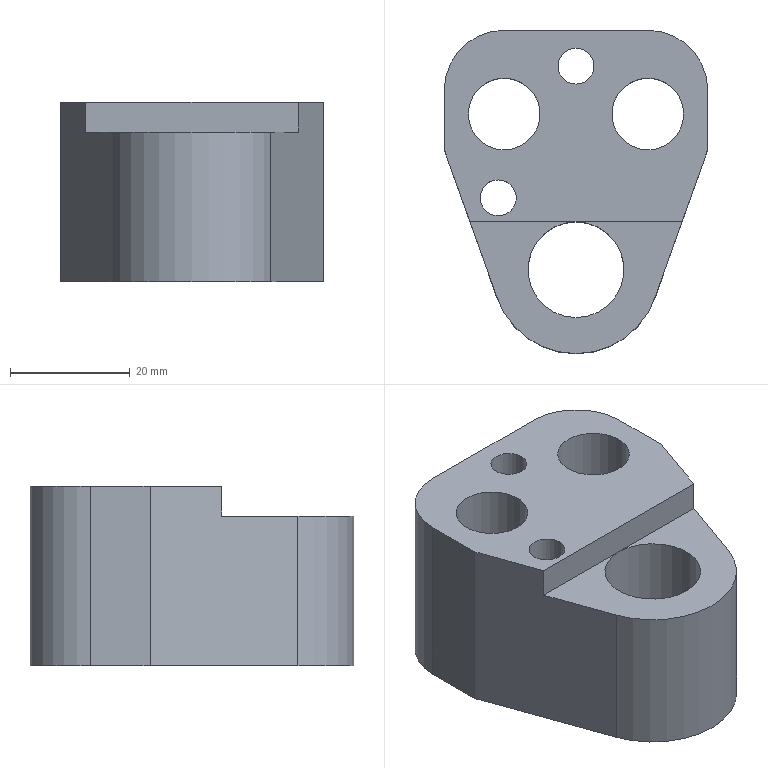Part | NX | features solid 2 | 1 solid | 25 faces | box 44 x 54 x 30 mm | volume 36572 mm3 | plane 13 | cylinder 12 | commonest cylinder face diameters 6 x2 8 x2 12 x2 17 x2 20 x2 16 x1
STEP:
#1=CARTESIAN_POINT('',(278.65,-40.99,61.));
#2=VERTEX_POINT('',#1);
#3=CARTESIAN_POINT('',(278.65,-36.99,61.));
#4=DIRECTION('',(0.,0.,1.));
#5=DIRECTION('',(0.,-1.,0.));
#6=AXIS2_PLACEMENT_3D('',#3,#4,#5);
#7=CIRCLE('',#6,4.);
#8=EDGE_CURVE('',#2,#2,#7,.F.);
#9=ORIENTED_EDGE('',*,*,#8,.F.);
#10=EDGE_LOOP('',(#9));
#11=FACE_BOUND('',#10,.T.);
#12=CARTESIAN_POINT('',(266.65,-36.49,61.));
#13=VERTEX_POINT('',#12);
#14=CARTESIAN_POINT('',(266.65,-44.99,61.));
#15=DIRECTION('',(0.,0.,-1.));
#16=DIRECTION('',(0.,1.,0.));
#17=AXIS2_PLACEMENT_3D('',#14,#15,#16);
#18=CIRCLE('',#17,8.5);
#19=EDGE_CURVE('',#13,#13,#18,.T.);
#20=ORIENTED_EDGE('',*,*,#19,.F.);
#21=EDGE_LOOP('',(#20));
#22=FACE_BOUND('',#21,.T.);
#23=CARTESIAN_POINT('',(290.65,-36.49,61.));
#24=VERTEX_POINT('',#23);
#25=CARTESIAN_POINT('',(290.65,-44.99,61.));
#26=DIRECTION('',(0.,0.,-1.));
#27=DIRECTION('',(0.,1.,0.));
#28=AXIS2_PLACEMENT_3D('',#25,#26,#27);
#29=CIRCLE('',#28,8.5);
#30=EDGE_CURVE('',#24,#24,#29,.T.);
#31=ORIENTED_EDGE('',*,*,#30,.F.);
#32=EDGE_LOOP('',(#31));
#33=FACE_BOUND('',#32,.T.);
#34=CARTESIAN_POINT('',(278.65,-78.99,61.));
#35=VERTEX_POINT('',#34);
#36=CARTESIAN_POINT('',(278.65,-70.99,61.));
#37=DIRECTION('',(0.,0.,1.));
#38=DIRECTION('',(0.,-1.,0.));
#39=AXIS2_PLACEMENT_3D('',#36,#37,#38);
#40=CIRCLE('',#39,8.);
#41=EDGE_CURVE('',#35,#35,#40,.T.);
#42=ORIENTED_EDGE('',*,*,#41,.T.);
#43=EDGE_LOOP('',(#42));
#44=FACE_BOUND('',#43,.T.);
#45=CARTESIAN_POINT('',(291.836,-75.694,61.));
#46=VERTEX_POINT('',#45);
#47=CARTESIAN_POINT('',(300.65,-50.99,61.));
#48=VERTEX_POINT('',#47);
#49=CARTESIAN_POINT('',(291.836,-75.694,61.));
#50=DIRECTION('',(0.336,0.9418,0.));
#51=VECTOR('',#50,1000.);
#52=LINE('',#49,#51);
#53=EDGE_CURVE('',#46,#48,#52,.T.);
#54=ORIENTED_EDGE('',*,*,#53,.F.);
#55=CARTESIAN_POINT('',(265.464,-75.694,61.));
#56=VERTEX_POINT('',#55);
#57=CARTESIAN_POINT('',(278.65,-70.99,61.));
#58=DIRECTION('',(0.,0.,-1.));
#59=DIRECTION('',(0.,1.,0.));
#60=AXIS2_PLACEMENT_3D('',#57,#58,#59);
#61=CIRCLE('',#60,14.);
#62=EDGE_CURVE('',#46,#56,#61,.T.);
#63=ORIENTED_EDGE('',*,*,#62,.T.);
#64=CARTESIAN_POINT('',(256.65,-50.99,61.));
#65=VERTEX_POINT('',#64);
#66=CARTESIAN_POINT('',(265.464,-75.694,61.));
#67=DIRECTION('',(-0.336,0.9418,0.));
#68=VECTOR('',#67,1000.);
#69=LINE('',#66,#68);
#70=EDGE_CURVE('',#56,#65,#69,.T.);
#71=ORIENTED_EDGE('',*,*,#70,.T.);
#72=CARTESIAN_POINT('',(256.65,-40.99,61.));
#73=VERTEX_POINT('',#72);
#74=CARTESIAN_POINT('',(256.65,-50.99,61.));
#75=DIRECTION('',(0.,1.,0.));
#76=VECTOR('',#75,1000.);
#77=LINE('',#74,#76);
#78=EDGE_CURVE('',#65,#73,#77,.T.);
#79=ORIENTED_EDGE('',*,*,#78,.T.);
#80=CARTESIAN_POINT('',(266.65,-30.99,61.));
#81=VERTEX_POINT('',#80);
#82=CARTESIAN_POINT('',(266.65,-40.99,61.));
#83=DIRECTION('',(0.,0.,-1.));
#84=DIRECTION('',(0.,1.,0.));
#85=AXIS2_PLACEMENT_3D('',#82,#83,#84);
#86=CIRCLE('',#85,10.);
#87=EDGE_CURVE('',#73,#81,#86,.T.);
#88=ORIENTED_EDGE('',*,*,#87,.T.);
#89=CARTESIAN_POINT('',(290.65,-30.99,61.));
#90=VERTEX_POINT('',#89);
#91=CARTESIAN_POINT('',(290.65,-30.99,61.));
#92=DIRECTION('',(-1.,0.,0.));
#93=VECTOR('',#92,1000.);
#94=LINE('',#91,#93);
#95=EDGE_CURVE('',#90,#81,#94,.T.);
#96=ORIENTED_EDGE('',*,*,#95,.F.);
#97=CARTESIAN_POINT('',(300.65,-40.99,61.));
#98=VERTEX_POINT('',#97);
#99=CARTESIAN_POINT('',(290.65,-40.99,61.));
#100=DIRECTION('',(0.,0.,-1.));
#101=DIRECTION('',(0.,1.,0.));
#102=AXIS2_PLACEMENT_3D('',#99,#100,#101);
#103=CIRCLE('',#102,10.);
#104=EDGE_CURVE('',#90,#98,#103,.T.);
#105=ORIENTED_EDGE('',*,*,#104,.T.);
#106=CARTESIAN_POINT('',(300.65,-50.99,61.));
#107=DIRECTION('',(0.,1.,0.));
#108=VECTOR('',#107,1000.);
#109=LINE('',#106,#108);
#110=EDGE_CURVE('',#48,#98,#109,.T.);
#111=ORIENTED_EDGE('',*,*,#110,.F.);
#112=EDGE_LOOP('',(#54,#63,#71,#79,#88,#96,#105,#111));
#113=FACE_BOUND('',#112,.T.);
#114=CARTESIAN_POINT('',(265.65,-62.99,61.));
#115=VERTEX_POINT('',#114);
#116=CARTESIAN_POINT('',(265.65,-58.99,61.));
#117=DIRECTION('',(0.,0.,1.));
#118=DIRECTION('',(0.,-1.,0.));
#119=AXIS2_PLACEMENT_3D('',#116,#117,#118);
#120=CIRCLE('',#119,4.);
#121=EDGE_CURVE('',#115,#115,#120,.F.);
#122=ORIENTED_EDGE('',*,*,#121,.F.);
#123=EDGE_LOOP('',(#122));
#124=FACE_BOUND('',#123,.T.);
#125=CARTESIAN_POINT('',(290.65,-40.99,61.));
#126=DIRECTION('',(0.,0.,-1.));
#127=DIRECTION('',(0.,1.,0.));
#128=AXIS2_PLACEMENT_3D('',#125,#126,#127);
#129=PLANE('',#128);
#130=ADVANCED_FACE('',(#11,#22,#33,#44,#113,#124),#129,.T.);
#131=CARTESIAN_POINT('',(278.65,-33.99,91.));
#132=VERTEX_POINT('',#131);
#133=CARTESIAN_POINT('',(278.65,-36.99,91.));
#134=DIRECTION('',(0.,0.,-1.));
#135=DIRECTION('',(0.,1.,0.));
#136=AXIS2_PLACEMENT_3D('',#133,#134,#135);
#137=CIRCLE('',#136,3.);
#138=EDGE_CURVE('',#132,#132,#137,.T.);
#139=ORIENTED_EDGE('',*,*,#138,.F.);
#140=EDGE_LOOP('',(#139));
#141=FACE_BOUND('',#140,.T.);
#142=CARTESIAN_POINT('',(278.65,-33.99,81.));
#143=VERTEX_POINT('',#142);
#144=CARTESIAN_POINT('',(278.65,-36.99,81.));
#145=DIRECTION('',(0.,0.,-1.));
#146=DIRECTION('',(0.,1.,0.));
#147=AXIS2_PLACEMENT_3D('',#144,#145,#146);
#148=CIRCLE('',#147,3.);
#149=EDGE_CURVE('',#143,#143,#148,.T.);
#150=ORIENTED_EDGE('',*,*,#149,.T.);
#151=EDGE_LOOP('',(#150));
#152=FACE_BOUND('',#151,.T.);
#153=CARTESIAN_POINT('',(278.65,-36.99,61.));
#154=DIRECTION('',(0.,0.,1.));
#155=DIRECTION('',(0.,-1.,0.));
#156=AXIS2_PLACEMENT_3D('',#153,#154,#155);
#157=CYLINDRICAL_SURFACE('',#156,3.);
#158=ADVANCED_FACE('',(#141,#152),#157,.F.);
#159=CARTESIAN_POINT('',(266.65,-38.99,91.));
#160=VERTEX_POINT('',#159);
#161=CARTESIAN_POINT('',(266.65,-44.99,91.));
#162=DIRECTION('',(0.,0.,-1.));
#163=DIRECTION('',(0.,1.,0.));
#164=AXIS2_PLACEMENT_3D('',#161,#162,#163);
#165=CIRCLE('',#164,6.);
#166=EDGE_CURVE('',#160,#160,#165,.T.);
#167=ORIENTED_EDGE('',*,*,#166,.F.);
#168=EDGE_LOOP('',(#167));
#169=FACE_BOUND('',#168,.T.);
#170=CARTESIAN_POINT('',(266.65,-38.99,73.));
#171=VERTEX_POINT('',#170);
#172=CARTESIAN_POINT('',(266.65,-44.99,73.));
#173=DIRECTION('',(0.,0.,-1.));
#174=DIRECTION('',(0.,1.,0.));
#175=AXIS2_PLACEMENT_3D('',#172,#173,#174);
#176=CIRCLE('',#175,6.);
#177=EDGE_CURVE('',#171,#171,#176,.T.);
#178=ORIENTED_EDGE('',*,*,#177,.T.);
#179=EDGE_LOOP('',(#178));
#180=FACE_BOUND('',#179,.T.);
#181=CARTESIAN_POINT('',(266.65,-44.99,61.));
#182=DIRECTION('',(0.,0.,1.));
#183=DIRECTION('',(0.,-1.,0.));
#184=AXIS2_PLACEMENT_3D('',#181,#182,#183);
#185=CYLINDRICAL_SURFACE('',#184,6.);
#186=ADVANCED_FACE('',(#169,#180),#185,.F.);
#187=CARTESIAN_POINT('',(290.65,-38.99,91.));
#188=VERTEX_POINT('',#187);
#189=CARTESIAN_POINT('',(290.65,-44.99,91.));
#190=DIRECTION('',(0.,0.,-1.));
#191=DIRECTION('',(0.,1.,0.));
#192=AXIS2_PLACEMENT_3D('',#189,#190,#191);
#193=CIRCLE('',#192,6.);
#194=EDGE_CURVE('',#188,#188,#193,.T.);
#195=ORIENTED_EDGE('',*,*,#194,.F.);
#196=EDGE_LOOP('',(#195));
#197=FACE_BOUND('',#196,.T.);
#198=CARTESIAN_POINT('',(290.65,-38.99,73.));
#199=VERTEX_POINT('',#198);
#200=CARTESIAN_POINT('',(290.65,-44.99,73.));
#201=DIRECTION('',(0.,0.,-1.));
#202=DIRECTION('',(0.,1.,0.));
#203=AXIS2_PLACEMENT_3D('',#200,#201,#202);
#204=CIRCLE('',#203,6.);
#205=EDGE_CURVE('',#199,#199,#204,.T.);
#206=ORIENTED_EDGE('',*,*,#205,.T.);
#207=EDGE_LOOP('',(#206));
#208=FACE_BOUND('',#207,.T.);
#209=CARTESIAN_POINT('',(290.65,-44.99,61.));
#210=DIRECTION('',(0.,0.,1.));
#211=DIRECTION('',(0.,-1.,0.));
#212=AXIS2_PLACEMENT_3D('',#209,#210,#211);
#213=CYLINDRICAL_SURFACE('',#212,6.);
#214=ADVANCED_FACE('',(#197,#208),#213,.F.);
#215=CARTESIAN_POINT('',(265.65,-55.99,91.));
#216=VERTEX_POINT('',#215);
#217=CARTESIAN_POINT('',(265.65,-58.99,91.));
#218=DIRECTION('',(0.,0.,-1.));
#219=DIRECTION('',(0.,1.,0.));
#220=AXIS2_PLACEMENT_3D('',#217,#218,#219);
#221=CIRCLE('',#220,3.);
#222=EDGE_CURVE('',#216,#216,#221,.T.);
#223=ORIENTED_EDGE('',*,*,#222,.T.);
#224=EDGE_LOOP('',(#223));
#225=FACE_BOUND('',#224,.T.);
#226=ORIENTED_EDGE('',*,*,#166,.T.);
#227=EDGE_LOOP('',(#226));
#228=FACE_BOUND('',#227,.T.);
#229=CARTESIAN_POINT('',(260.931,-62.99,91.));
#230=VERTEX_POINT('',#229);
#231=CARTESIAN_POINT('',(256.65,-50.99,91.));
#232=VERTEX_POINT('',#231);
#233=CARTESIAN_POINT('',(265.464,-75.694,91.));
#234=DIRECTION('',(-0.336,0.9418,0.));
#235=VECTOR('',#234,1000.);
#236=LINE('',#233,#235);
#237=EDGE_CURVE('',#230,#232,#236,.T.);
#238=ORIENTED_EDGE('',*,*,#237,.F.);
#239=CARTESIAN_POINT('',(296.368,-62.99,91.));
#240=VERTEX_POINT('',#239);
#241=CARTESIAN_POINT('',(296.368,-62.99,91.));
#242=DIRECTION('',(-1.,0.,0.));
#243=VECTOR('',#242,1000.);
#244=LINE('',#241,#243);
#245=EDGE_CURVE('',#240,#230,#244,.T.);
#246=ORIENTED_EDGE('',*,*,#245,.F.);
#247=CARTESIAN_POINT('',(300.65,-50.99,91.));
#248=VERTEX_POINT('',#247);
#249=CARTESIAN_POINT('',(291.836,-75.694,91.));
#250=DIRECTION('',(0.336,0.9418,0.));
#251=VECTOR('',#250,1000.);
#252=LINE('',#249,#251);
#253=EDGE_CURVE('',#240,#248,#252,.T.);
#254=ORIENTED_EDGE('',*,*,#253,.T.);
#255=CARTESIAN_POINT('',(300.65,-40.99,91.));
#256=VERTEX_POINT('',#255);
#257=CARTESIAN_POINT('',(300.65,-50.99,91.));
#258=DIRECTION('',(0.,1.,0.));
#259=VECTOR('',#258,1000.);
#260=LINE('',#257,#259);
#261=EDGE_CURVE('',#248,#256,#260,.T.);
#262=ORIENTED_EDGE('',*,*,#261,.T.);
#263=CARTESIAN_POINT('',(290.65,-30.99,91.));
#264=VERTEX_POINT('',#263);
#265=CARTESIAN_POINT('',(290.65,-40.99,91.));
#266=DIRECTION('',(0.,0.,-1.));
#267=DIRECTION('',(0.,1.,0.));
#268=AXIS2_PLACEMENT_3D('',#265,#266,#267);
#269=CIRCLE('',#268,10.);
#270=EDGE_CURVE('',#264,#256,#269,.T.);
#271=ORIENTED_EDGE('',*,*,#270,.F.);
#272=CARTESIAN_POINT('',(266.65,-30.99,91.));
#273=VERTEX_POINT('',#272);
#274=CARTESIAN_POINT('',(290.65,-30.99,91.));
#275=DIRECTION('',(-1.,0.,0.));
#276=VECTOR('',#275,1000.);
#277=LINE('',#274,#276);
#278=EDGE_CURVE('',#264,#273,#277,.T.);
#279=ORIENTED_EDGE('',*,*,#278,.T.);
#280=CARTESIAN_POINT('',(256.65,-40.99,91.));
#281=VERTEX_POINT('',#280);
#282=CARTESIAN_POINT('',(266.65,-40.99,91.));
#283=DIRECTION('',(0.,0.,-1.));
#284=DIRECTION('',(0.,1.,0.));
#285=AXIS2_PLACEMENT_3D('',#282,#283,#284);
#286=CIRCLE('',#285,10.);
#287=EDGE_CURVE('',#281,#273,#286,.T.);
#288=ORIENTED_EDGE('',*,*,#287,.F.);
#289=CARTESIAN_POINT('',(256.65,-50.99,91.));
#290=DIRECTION('',(0.,1.,0.));
#291=VECTOR('',#290,1000.);
#292=LINE('',#289,#291);
#293=EDGE_CURVE('',#232,#281,#292,.T.);
#294=ORIENTED_EDGE('',*,*,#293,.F.);
#295=EDGE_LOOP('',(#238,#246,#254,#262,#271,#279,#288,#294));
#296=FACE_BOUND('',#295,.T.);
#297=ORIENTED_EDGE('',*,*,#194,.T.);
#298=EDGE_LOOP('',(#297));
#299=FACE_BOUND('',#298,.T.);
#300=ORIENTED_EDGE('',*,*,#138,.T.);
#301=EDGE_LOOP('',(#300));
#302=FACE_BOUND('',#301,.T.);
#303=CARTESIAN_POINT('',(290.65,-40.99,91.));
#304=DIRECTION('',(0.,0.,-1.));
#305=DIRECTION('',(0.,1.,0.));
#306=AXIS2_PLACEMENT_3D('',#303,#304,#305);
#307=PLANE('',#306);
#308=ADVANCED_FACE('',(#225,#228,#296,#299,#302),#307,.F.);
#309=CARTESIAN_POINT('',(296.368,-62.99,86.));
#310=VERTEX_POINT('',#309);
#311=CARTESIAN_POINT('',(296.368,-62.99,86.));
#312=DIRECTION('',(0.,0.,1.));
#313=VECTOR('',#312,1000.);
#314=LINE('',#311,#313);
#315=EDGE_CURVE('',#310,#240,#314,.T.);
#316=ORIENTED_EDGE('',*,*,#315,.F.);
#317=CARTESIAN_POINT('',(291.836,-75.694,86.));
#318=VERTEX_POINT('',#317);
#319=CARTESIAN_POINT('',(296.368,-62.99,86.));
#320=DIRECTION('',(-0.336,-0.9418,0.));
#321=VECTOR('',#320,1000.);
#322=LINE('',#319,#321);
#323=EDGE_CURVE('',#310,#318,#322,.T.);
#324=ORIENTED_EDGE('',*,*,#323,.T.);
#325=CARTESIAN_POINT('',(291.836,-75.694,61.));
#326=DIRECTION('',(0.,0.,1.));
#327=VECTOR('',#326,1000.);
#328=LINE('',#325,#327);
#329=EDGE_CURVE('',#46,#318,#328,.T.);
#330=ORIENTED_EDGE('',*,*,#329,.F.);
#331=ORIENTED_EDGE('',*,*,#53,.T.);
#332=CARTESIAN_POINT('',(300.65,-50.99,61.));
#333=DIRECTION('',(0.,0.,1.));
#334=VECTOR('',#333,1000.);
#335=LINE('',#332,#334);
#336=EDGE_CURVE('',#48,#248,#335,.T.);
#337=ORIENTED_EDGE('',*,*,#336,.T.);
#338=ORIENTED_EDGE('',*,*,#253,.F.);
#339=EDGE_LOOP('',(#316,#324,#330,#331,#337,#338));
#340=FACE_BOUND('',#339,.T.);
#341=CARTESIAN_POINT('',(291.836,-75.694,61.));
#342=DIRECTION('',(0.9418,-0.336,0.));
#343=DIRECTION('',(0.336,0.9418,0.));
#344=AXIS2_PLACEMENT_3D('',#341,#342,#343);
#345=PLANE('',#344);
#346=ADVANCED_FACE('',(#340),#345,.T.);
#347=ORIENTED_EDGE('',*,*,#261,.F.);
#348=ORIENTED_EDGE('',*,*,#336,.F.);
#349=ORIENTED_EDGE('',*,*,#110,.T.);
#350=CARTESIAN_POINT('',(300.65,-40.99,61.));
#351=DIRECTION('',(0.,0.,1.));
#352=VECTOR('',#351,1000.);
#353=LINE('',#350,#352);
#354=EDGE_CURVE('',#98,#256,#353,.T.);
#355=ORIENTED_EDGE('',*,*,#354,.T.);
#356=EDGE_LOOP('',(#347,#348,#349,#355));
#357=FACE_BOUND('',#356,.T.);
#358=CARTESIAN_POINT('',(300.65,-50.99,61.));
#359=DIRECTION('',(1.,0.,0.));
#360=DIRECTION('',(0.,0.,1.));
#361=AXIS2_PLACEMENT_3D('',#358,#359,#360);
#362=PLANE('',#361);
#363=ADVANCED_FACE('',(#357),#362,.T.);
#364=ORIENTED_EDGE('',*,*,#270,.T.);
#365=ORIENTED_EDGE('',*,*,#354,.F.);
#366=ORIENTED_EDGE('',*,*,#104,.F.);
#367=CARTESIAN_POINT('',(290.65,-30.99,61.));
#368=DIRECTION('',(0.,0.,1.));
#369=VECTOR('',#368,1000.);
#370=LINE('',#367,#369);
#371=EDGE_CURVE('',#90,#264,#370,.T.);
#372=ORIENTED_EDGE('',*,*,#371,.T.);
#373=EDGE_LOOP('',(#364,#365,#366,#372));
#374=FACE_BOUND('',#373,.T.);
#375=CARTESIAN_POINT('',(290.65,-40.99,61.));
#376=DIRECTION('',(0.,0.,1.));
#377=DIRECTION('',(0.,-1.,0.));
#378=AXIS2_PLACEMENT_3D('',#375,#376,#377);
#379=CYLINDRICAL_SURFACE('',#378,10.);
#380=ADVANCED_FACE('',(#374),#379,.T.);
#381=ORIENTED_EDGE('',*,*,#278,.F.);
#382=ORIENTED_EDGE('',*,*,#371,.F.);
#383=ORIENTED_EDGE('',*,*,#95,.T.);
#384=CARTESIAN_POINT('',(266.65,-30.99,61.));
#385=DIRECTION('',(0.,0.,1.));
#386=VECTOR('',#385,1000.);
#387=LINE('',#384,#386);
#388=EDGE_CURVE('',#81,#273,#387,.T.);
#389=ORIENTED_EDGE('',*,*,#388,.T.);
#390=EDGE_LOOP('',(#381,#382,#383,#389));
#391=FACE_BOUND('',#390,.T.);
#392=CARTESIAN_POINT('',(290.65,-30.99,61.));
#393=DIRECTION('',(0.,1.,0.));
#394=DIRECTION('',(-1.,0.,0.));
#395=AXIS2_PLACEMENT_3D('',#392,#393,#394);
#396=PLANE('',#395);
#397=ADVANCED_FACE('',(#391),#396,.T.);
#398=ORIENTED_EDGE('',*,*,#287,.T.);
#399=ORIENTED_EDGE('',*,*,#388,.F.);
#400=ORIENTED_EDGE('',*,*,#87,.F.);
#401=CARTESIAN_POINT('',(256.65,-40.99,61.));
#402=DIRECTION('',(0.,0.,1.));
#403=VECTOR('',#402,1000.);
#404=LINE('',#401,#403);
#405=EDGE_CURVE('',#73,#281,#404,.T.);
#406=ORIENTED_EDGE('',*,*,#405,.T.);
#407=EDGE_LOOP('',(#398,#399,#400,#406));
#408=FACE_BOUND('',#407,.T.);
#409=CARTESIAN_POINT('',(266.65,-40.99,61.));
#410=DIRECTION('',(0.,0.,1.));
#411=DIRECTION('',(0.,-1.,0.));
#412=AXIS2_PLACEMENT_3D('',#409,#410,#411);
#413=CYLINDRICAL_SURFACE('',#412,10.);
#414=ADVANCED_FACE('',(#408),#413,.T.);
#415=ORIENTED_EDGE('',*,*,#293,.T.);
#416=ORIENTED_EDGE('',*,*,#405,.F.);
#417=ORIENTED_EDGE('',*,*,#78,.F.);
#418=CARTESIAN_POINT('',(256.65,-50.99,61.));
#419=DIRECTION('',(0.,0.,1.));
#420=VECTOR('',#419,1000.);
#421=LINE('',#418,#420);
#422=EDGE_CURVE('',#65,#232,#421,.T.);
#423=ORIENTED_EDGE('',*,*,#422,.T.);
#424=EDGE_LOOP('',(#415,#416,#417,#423));
#425=FACE_BOUND('',#424,.T.);
#426=CARTESIAN_POINT('',(256.65,-50.99,61.));
#427=DIRECTION('',(1.,0.,0.));
#428=DIRECTION('',(0.,0.,1.));
#429=AXIS2_PLACEMENT_3D('',#426,#427,#428);
#430=PLANE('',#429);
#431=ADVANCED_FACE('',(#425),#430,.F.);
#432=CARTESIAN_POINT('',(260.931,-62.99,86.));
#433=VERTEX_POINT('',#432);
#434=CARTESIAN_POINT('',(265.464,-75.694,86.));
#435=VERTEX_POINT('',#434);
#436=CARTESIAN_POINT('',(260.931,-62.99,86.));
#437=DIRECTION('',(0.336,-0.9418,0.));
#438=VECTOR('',#437,1000.);
#439=LINE('',#436,#438);
#440=EDGE_CURVE('',#433,#435,#439,.T.);
#441=ORIENTED_EDGE('',*,*,#440,.F.);
#442=CARTESIAN_POINT('',(260.931,-62.99,86.));
#443=DIRECTION('',(0.,0.,1.));
#444=VECTOR('',#443,1000.);
#445=LINE('',#442,#444);
#446=EDGE_CURVE('',#433,#230,#445,.T.);
#447=ORIENTED_EDGE('',*,*,#446,.T.);
#448=ORIENTED_EDGE('',*,*,#237,.T.);
#449=ORIENTED_EDGE('',*,*,#422,.F.);
#450=ORIENTED_EDGE('',*,*,#70,.F.);
#451=CARTESIAN_POINT('',(265.464,-75.694,61.));
#452=DIRECTION('',(0.,0.,1.));
#453=VECTOR('',#452,1000.);
#454=LINE('',#451,#453);
#455=EDGE_CURVE('',#56,#435,#454,.T.);
#456=ORIENTED_EDGE('',*,*,#455,.T.);
#457=EDGE_LOOP('',(#441,#447,#448,#449,#450,#456));
#458=FACE_BOUND('',#457,.T.);
#459=CARTESIAN_POINT('',(265.464,-75.694,61.));
#460=DIRECTION('',(0.9418,0.336,0.));
#461=DIRECTION('',(-0.336,0.9418,0.));
#462=AXIS2_PLACEMENT_3D('',#459,#460,#461);
#463=PLANE('',#462);
#464=ADVANCED_FACE('',(#458),#463,.F.);
#465=ORIENTED_EDGE('',*,*,#329,.T.);
#466=CARTESIAN_POINT('',(278.65,-70.99,86.));
#467=DIRECTION('',(0.,0.,-1.));
#468=DIRECTION('',(0.,1.,0.));
#469=AXIS2_PLACEMENT_3D('',#466,#467,#468);
#470=CIRCLE('',#469,14.);
#471=EDGE_CURVE('',#318,#435,#470,.T.);
#472=ORIENTED_EDGE('',*,*,#471,.T.);
#473=ORIENTED_EDGE('',*,*,#455,.F.);
#474=ORIENTED_EDGE('',*,*,#62,.F.);
#475=EDGE_LOOP('',(#465,#472,#473,#474));
#476=FACE_BOUND('',#475,.T.);
#477=CARTESIAN_POINT('',(278.65,-70.99,61.));
#478=DIRECTION('',(0.,0.,1.));
#479=DIRECTION('',(0.,-1.,0.));
#480=AXIS2_PLACEMENT_3D('',#477,#478,#479);
#481=CYLINDRICAL_SURFACE('',#480,14.);
#482=ADVANCED_FACE('',(#476),#481,.T.);
#483=CARTESIAN_POINT('',(278.65,-62.99,86.));
#484=VERTEX_POINT('',#483);
#485=CARTESIAN_POINT('',(278.65,-70.99,86.));
#486=DIRECTION('',(0.,0.,-1.));
#487=DIRECTION('',(0.,1.,0.));
#488=AXIS2_PLACEMENT_3D('',#485,#486,#487);
#489=CIRCLE('',#488,8.);
#490=EDGE_CURVE('',#484,#484,#489,.F.);
#491=ORIENTED_EDGE('',*,*,#490,.T.);
#492=EDGE_LOOP('',(#491));
#493=FACE_BOUND('',#492,.T.);
#494=ORIENTED_EDGE('',*,*,#41,.F.);
#495=EDGE_LOOP('',(#494));
#496=FACE_BOUND('',#495,.T.);
#497=CARTESIAN_POINT('',(278.65,-70.99,61.));
#498=DIRECTION('',(0.,0.,1.));
#499=DIRECTION('',(0.,-1.,0.));
#500=AXIS2_PLACEMENT_3D('',#497,#498,#499);
#501=CYLINDRICAL_SURFACE('',#500,8.);
#502=ADVANCED_FACE('',(#493,#496),#501,.F.);
#503=ORIENTED_EDGE('',*,*,#245,.T.);
#504=ORIENTED_EDGE('',*,*,#446,.F.);
#505=CARTESIAN_POINT('',(296.368,-62.99,86.));
#506=DIRECTION('',(-1.,0.,0.));
#507=VECTOR('',#506,1000.);
#508=LINE('',#505,#507);
#509=EDGE_CURVE('',#484,#433,#508,.T.);
#510=ORIENTED_EDGE('',*,*,#509,.F.);
#511=CARTESIAN_POINT('',(296.368,-62.99,86.));
#512=DIRECTION('',(-1.,0.,0.));
#513=VECTOR('',#512,1000.);
#514=LINE('',#511,#513);
#515=EDGE_CURVE('',#310,#484,#514,.T.);
#516=ORIENTED_EDGE('',*,*,#515,.F.);
#517=ORIENTED_EDGE('',*,*,#315,.T.);
#518=EDGE_LOOP('',(#503,#504,#510,#516,#517));
#519=FACE_BOUND('',#518,.T.);
#520=CARTESIAN_POINT('',(296.368,-62.99,86.));
#521=DIRECTION('',(0.,1.,0.));
#522=DIRECTION('',(-1.,0.,0.));
#523=AXIS2_PLACEMENT_3D('',#520,#521,#522);
#524=PLANE('',#523);
#525=ADVANCED_FACE('',(#519),#524,.F.);
#526=ORIENTED_EDGE('',*,*,#509,.T.);
#527=ORIENTED_EDGE('',*,*,#440,.T.);
#528=ORIENTED_EDGE('',*,*,#471,.F.);
#529=ORIENTED_EDGE('',*,*,#323,.F.);
#530=ORIENTED_EDGE('',*,*,#515,.T.);
#531=ORIENTED_EDGE('',*,*,#490,.F.);
#532=EDGE_LOOP('',(#526,#527,#528,#529,#530,#531));
#533=FACE_BOUND('',#532,.T.);
#534=CARTESIAN_POINT('',(278.65,-70.99,86.));
#535=DIRECTION('',(0.,0.,-1.));
#536=DIRECTION('',(0.,1.,0.));
#537=AXIS2_PLACEMENT_3D('',#534,#535,#536);
#538=PLANE('',#537);
#539=ADVANCED_FACE('',(#533),#538,.F.);
#540=CARTESIAN_POINT('',(265.65,-55.99,81.));
#541=VERTEX_POINT('',#540);
#542=CARTESIAN_POINT('',(265.65,-58.99,81.));
#543=DIRECTION('',(0.,0.,-1.));
#544=DIRECTION('',(0.,1.,0.));
#545=AXIS2_PLACEMENT_3D('',#542,#543,#544);
#546=CIRCLE('',#545,3.);
#547=EDGE_CURVE('',#541,#541,#546,.T.);
#548=ORIENTED_EDGE('',*,*,#547,.T.);
#549=EDGE_LOOP('',(#548));
#550=FACE_BOUND('',#549,.T.);
#551=ORIENTED_EDGE('',*,*,#222,.F.);
#552=EDGE_LOOP('',(#551));
#553=FACE_BOUND('',#552,.T.);
#554=CARTESIAN_POINT('',(265.65,-58.99,61.));
#555=DIRECTION('',(0.,0.,1.));
#556=DIRECTION('',(0.,-1.,0.));
#557=AXIS2_PLACEMENT_3D('',#554,#555,#556);
#558=CYLINDRICAL_SURFACE('',#557,3.);
#559=ADVANCED_FACE('',(#550,#553),#558,.F.);
#560=CARTESIAN_POINT('',(290.65,-36.49,73.));
#561=VERTEX_POINT('',#560);
#562=CARTESIAN_POINT('',(290.65,-44.99,73.));
#563=DIRECTION('',(0.,0.,-1.));
#564=DIRECTION('',(0.,1.,0.));
#565=AXIS2_PLACEMENT_3D('',#562,#563,#564);
#566=CIRCLE('',#565,8.5);
#567=EDGE_CURVE('',#561,#561,#566,.T.);
#568=ORIENTED_EDGE('',*,*,#567,.F.);
#569=EDGE_LOOP('',(#568));
#570=FACE_BOUND('',#569,.T.);
#571=ORIENTED_EDGE('',*,*,#30,.T.);
#572=EDGE_LOOP('',(#571));
#573=FACE_BOUND('',#572,.T.);
#574=CARTESIAN_POINT('',(290.65,-44.99,73.));
#575=DIRECTION('',(0.,0.,-1.));
#576=DIRECTION('',(0.,1.,0.));
#577=AXIS2_PLACEMENT_3D('',#574,#575,#576);
#578=CYLINDRICAL_SURFACE('',#577,8.5);
#579=ADVANCED_FACE('',(#570,#573),#578,.F.);
#580=ORIENTED_EDGE('',*,*,#205,.F.);
#581=EDGE_LOOP('',(#580));
#582=FACE_BOUND('',#581,.T.);
#583=ORIENTED_EDGE('',*,*,#567,.T.);
#584=EDGE_LOOP('',(#583));
#585=FACE_BOUND('',#584,.T.);
#586=CARTESIAN_POINT('',(290.65,-44.99,73.));
#587=DIRECTION('',(0.,0.,-1.));
#588=DIRECTION('',(0.,1.,0.));
#589=AXIS2_PLACEMENT_3D('',#586,#587,#588);
#590=PLANE('',#589);
#591=ADVANCED_FACE('',(#582,#585),#590,.T.);
#592=CARTESIAN_POINT('',(266.65,-36.49,73.));
#593=VERTEX_POINT('',#592);
#594=CARTESIAN_POINT('',(266.65,-44.99,73.));
#595=DIRECTION('',(0.,0.,-1.));
#596=DIRECTION('',(0.,1.,0.));
#597=AXIS2_PLACEMENT_3D('',#594,#595,#596);
#598=CIRCLE('',#597,8.5);
#599=EDGE_CURVE('',#593,#593,#598,.T.);
#600=ORIENTED_EDGE('',*,*,#599,.F.);
#601=EDGE_LOOP('',(#600));
#602=FACE_BOUND('',#601,.T.);
#603=ORIENTED_EDGE('',*,*,#19,.T.);
#604=EDGE_LOOP('',(#603));
#605=FACE_BOUND('',#604,.T.);
#606=CARTESIAN_POINT('',(266.65,-44.99,73.));
#607=DIRECTION('',(0.,0.,-1.));
#608=DIRECTION('',(0.,1.,0.));
#609=AXIS2_PLACEMENT_3D('',#606,#607,#608);
#610=CYLINDRICAL_SURFACE('',#609,8.5);
#611=ADVANCED_FACE('',(#602,#605),#610,.F.);
#612=ORIENTED_EDGE('',*,*,#177,.F.);
#613=EDGE_LOOP('',(#612));
#614=FACE_BOUND('',#613,.T.);
#615=ORIENTED_EDGE('',*,*,#599,.T.);
#616=EDGE_LOOP('',(#615));
#617=FACE_BOUND('',#616,.T.);
#618=CARTESIAN_POINT('',(266.65,-44.99,73.));
#619=DIRECTION('',(0.,0.,-1.));
#620=DIRECTION('',(0.,1.,0.));
#621=AXIS2_PLACEMENT_3D('',#618,#619,#620);
#622=PLANE('',#621);
#623=ADVANCED_FACE('',(#614,#617),#622,.T.);
#624=ORIENTED_EDGE('',*,*,#149,.F.);
#625=EDGE_LOOP('',(#624));
#626=FACE_BOUND('',#625,.T.);
#627=CARTESIAN_POINT('',(278.65,-40.99,81.));
#628=VERTEX_POINT('',#627);
#629=CARTESIAN_POINT('',(278.65,-36.99,81.));
#630=DIRECTION('',(0.,0.,1.));
#631=DIRECTION('',(0.,-1.,0.));
#632=AXIS2_PLACEMENT_3D('',#629,#630,#631);
#633=CIRCLE('',#632,4.);
#634=EDGE_CURVE('',#628,#628,#633,.F.);
#635=ORIENTED_EDGE('',*,*,#634,.T.);
#636=EDGE_LOOP('',(#635));
#637=FACE_BOUND('',#636,.T.);
#638=CARTESIAN_POINT('',(278.65,-36.99,81.));
#639=DIRECTION('',(0.,0.,1.));
#640=DIRECTION('',(0.,-1.,0.));
#641=AXIS2_PLACEMENT_3D('',#638,#639,#640);
#642=PLANE('',#641);
#643=ADVANCED_FACE('',(#626,#637),#642,.F.);
#644=ORIENTED_EDGE('',*,*,#634,.F.);
#645=EDGE_LOOP('',(#644));
#646=FACE_BOUND('',#645,.T.);
#647=ORIENTED_EDGE('',*,*,#8,.T.);
#648=EDGE_LOOP('',(#647));
#649=FACE_BOUND('',#648,.T.);
#650=CARTESIAN_POINT('',(278.65,-36.99,61.));
#651=DIRECTION('',(0.,0.,1.));
#652=DIRECTION('',(0.,-1.,0.));
#653=AXIS2_PLACEMENT_3D('',#650,#651,#652);
#654=CYLINDRICAL_SURFACE('',#653,4.);
#655=ADVANCED_FACE('',(#646,#649),#654,.F.);
#656=ORIENTED_EDGE('',*,*,#547,.F.);
#657=EDGE_LOOP('',(#656));
#658=FACE_BOUND('',#657,.T.);
#659=CARTESIAN_POINT('',(265.65,-62.99,81.));
#660=VERTEX_POINT('',#659);
#661=CARTESIAN_POINT('',(265.65,-58.99,81.));
#662=DIRECTION('',(0.,0.,1.));
#663=DIRECTION('',(0.,-1.,0.));
#664=AXIS2_PLACEMENT_3D('',#661,#662,#663);
#665=CIRCLE('',#664,4.);
#666=EDGE_CURVE('',#660,#660,#665,.F.);
#667=ORIENTED_EDGE('',*,*,#666,.T.);
#668=EDGE_LOOP('',(#667));
#669=FACE_BOUND('',#668,.T.);
#670=CARTESIAN_POINT('',(265.65,-58.99,81.));
#671=DIRECTION('',(0.,0.,1.));
#672=DIRECTION('',(0.,-1.,0.));
#673=AXIS2_PLACEMENT_3D('',#670,#671,#672);
#674=PLANE('',#673);
#675=ADVANCED_FACE('',(#658,#669),#674,.F.);
#676=ORIENTED_EDGE('',*,*,#666,.F.);
#677=EDGE_LOOP('',(#676));
#678=FACE_BOUND('',#677,.T.);
#679=ORIENTED_EDGE('',*,*,#121,.T.);
#680=EDGE_LOOP('',(#679));
#681=FACE_BOUND('',#680,.T.);
#682=CARTESIAN_POINT('',(265.65,-58.99,61.));
#683=DIRECTION('',(0.,0.,1.));
#684=DIRECTION('',(0.,-1.,0.));
#685=AXIS2_PLACEMENT_3D('',#682,#683,#684);
#686=CYLINDRICAL_SURFACE('',#685,4.);
#687=ADVANCED_FACE('',(#678,#681),#686,.F.);
#688=CLOSED_SHELL('',(#130,#158,#186,#214,#308,#346,#363,#380,#397,#414,#431,#464,#482,#502,#525,#539,#559,#579,#591,#611,#623,#643,#655,#675,#687));
#689=MANIFOLD_SOLID_BREP('',#688);
#690=(LENGTH_UNIT()NAMED_UNIT(*)SI_UNIT(.MILLI.,.METRE.));
#691=UNCERTAINTY_MEASURE_WITH_UNIT(LENGTH_MEASURE(0.00001),#690,'','');
#692=(NAMED_UNIT(*)PLANE_ANGLE_UNIT()SI_UNIT($,.RADIAN.));
#693=(NAMED_UNIT(*)SI_UNIT($,.STERADIAN.)SOLID_ANGLE_UNIT());
#694=(GEOMETRIC_REPRESENTATION_CONTEXT(3)GLOBAL_UNCERTAINTY_ASSIGNED_CONTEXT((#691))GLOBAL_UNIT_ASSIGNED_CONTEXT((#690,#692,#693))REPRESENTATION_CONTEXT('',''));
#695=ADVANCED_BREP_SHAPE_REPRESENTATION('',(#689),#694);